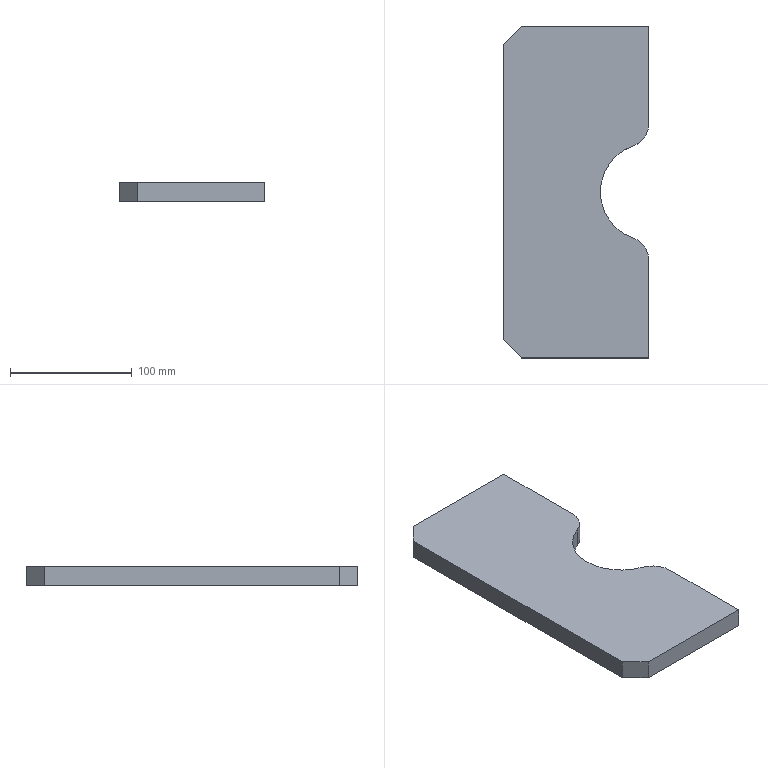Part | SolidWorks | features Extrusion 1 | 1 solid | 13 faces | box 120 x 273 x 16 mm | volume 478824 mm3 | plane 9 | cylinder 4 | commonest cylinder face diameters 40 x2 80 x2
STEP:
#1=CARTESIAN_POINT('',(80.,136.5,16.));
#2=VERTEX_POINT('',#1);
#3=CARTESIAN_POINT('',(106.667,174.212,16.));
#4=VERTEX_POINT('',#3);
#5=CARTESIAN_POINT('',(120.,136.5,16.));
#6=DIRECTION('',(0.,0.,-1.));
#7=DIRECTION('',(1.,0.,0.));
#8=AXIS2_PLACEMENT_3D('',#5,#6,#7);
#9=CIRCLE('',#8,40.);
#10=EDGE_CURVE('',#2,#4,#9,.T.);
#11=ORIENTED_EDGE('',*,*,#10,.F.);
#12=CARTESIAN_POINT('',(80.,136.5,0.));
#13=VERTEX_POINT('',#12);
#14=CARTESIAN_POINT('',(80.,136.5,16.));
#15=DIRECTION('',(0.,0.,-1.));
#16=VECTOR('',#15,1000.);
#17=LINE('',#14,#16);
#18=EDGE_CURVE('',#2,#13,#17,.T.);
#19=ORIENTED_EDGE('',*,*,#18,.T.);
#20=CARTESIAN_POINT('',(106.667,174.212,0.));
#21=VERTEX_POINT('',#20);
#22=CARTESIAN_POINT('',(120.,136.5,0.));
#23=DIRECTION('',(0.,0.,-1.));
#24=DIRECTION('',(1.,0.,0.));
#25=AXIS2_PLACEMENT_3D('',#22,#23,#24);
#26=CIRCLE('',#25,40.);
#27=EDGE_CURVE('',#13,#21,#26,.T.);
#28=ORIENTED_EDGE('',*,*,#27,.T.);
#29=CARTESIAN_POINT('',(106.667,174.212,16.));
#30=DIRECTION('',(0.,0.,-1.));
#31=VECTOR('',#30,1000.);
#32=LINE('',#29,#31);
#33=EDGE_CURVE('',#4,#21,#32,.T.);
#34=ORIENTED_EDGE('',*,*,#33,.F.);
#35=EDGE_LOOP('',(#11,#19,#28,#34));
#36=FACE_OUTER_BOUND('',#35,.T.);
#37=CARTESIAN_POINT('',(120.,136.5,16.));
#38=DIRECTION('',(0.,0.,-1.));
#39=DIRECTION('',(-1.,0.,0.));
#40=AXIS2_PLACEMENT_3D('',#37,#38,#39);
#41=CYLINDRICAL_SURFACE('',#40,40.);
#42=ADVANCED_FACE('',(#36),#41,.F.);
#43=CARTESIAN_POINT('',(120.,193.069,0.));
#44=VERTEX_POINT('',#43);
#45=CARTESIAN_POINT('',(120.,273.,0.));
#46=VERTEX_POINT('',#45);
#47=CARTESIAN_POINT('',(120.,193.069,0.));
#48=DIRECTION('',(0.,1.,0.));
#49=VECTOR('',#48,1000.);
#50=LINE('',#47,#49);
#51=EDGE_CURVE('',#44,#46,#50,.T.);
#52=ORIENTED_EDGE('',*,*,#51,.T.);
#53=CARTESIAN_POINT('',(120.,273.,16.));
#54=VERTEX_POINT('',#53);
#55=CARTESIAN_POINT('',(120.,273.,16.));
#56=DIRECTION('',(0.,0.,-1.));
#57=VECTOR('',#56,1000.);
#58=LINE('',#55,#57);
#59=EDGE_CURVE('',#54,#46,#58,.T.);
#60=ORIENTED_EDGE('',*,*,#59,.F.);
#61=CARTESIAN_POINT('',(120.,193.069,16.));
#62=VERTEX_POINT('',#61);
#63=CARTESIAN_POINT('',(120.,193.069,16.));
#64=DIRECTION('',(0.,1.,0.));
#65=VECTOR('',#64,1000.);
#66=LINE('',#63,#65);
#67=EDGE_CURVE('',#62,#54,#66,.T.);
#68=ORIENTED_EDGE('',*,*,#67,.F.);
#69=CARTESIAN_POINT('',(120.,193.069,16.));
#70=DIRECTION('',(0.,0.,-1.));
#71=VECTOR('',#70,1000.);
#72=LINE('',#69,#71);
#73=EDGE_CURVE('',#62,#44,#72,.T.);
#74=ORIENTED_EDGE('',*,*,#73,.T.);
#75=EDGE_LOOP('',(#52,#60,#68,#74));
#76=FACE_OUTER_BOUND('',#75,.T.);
#77=CARTESIAN_POINT('',(120.,193.069,16.));
#78=DIRECTION('',(-1.,0.,0.));
#79=DIRECTION('',(0.,0.,1.));
#80=AXIS2_PLACEMENT_3D('',#77,#78,#79);
#81=PLANE('',#80);
#82=ADVANCED_FACE('',(#76),#81,.F.);
#83=CARTESIAN_POINT('',(15.,273.,0.));
#84=VERTEX_POINT('',#83);
#85=CARTESIAN_POINT('',(15.,273.,0.));
#86=DIRECTION('',(-1.,0.,0.));
#87=VECTOR('',#86,1000.);
#88=LINE('',#85,#87);
#89=EDGE_CURVE('',#46,#84,#88,.T.);
#90=ORIENTED_EDGE('',*,*,#89,.T.);
#91=CARTESIAN_POINT('',(15.,273.,16.));
#92=VERTEX_POINT('',#91);
#93=CARTESIAN_POINT('',(15.,273.,16.));
#94=DIRECTION('',(0.,0.,-1.));
#95=VECTOR('',#94,1000.);
#96=LINE('',#93,#95);
#97=EDGE_CURVE('',#92,#84,#96,.T.);
#98=ORIENTED_EDGE('',*,*,#97,.F.);
#99=CARTESIAN_POINT('',(15.,273.,16.));
#100=DIRECTION('',(-1.,0.,0.));
#101=VECTOR('',#100,1000.);
#102=LINE('',#99,#101);
#103=EDGE_CURVE('',#54,#92,#102,.T.);
#104=ORIENTED_EDGE('',*,*,#103,.F.);
#105=ORIENTED_EDGE('',*,*,#59,.T.);
#106=EDGE_LOOP('',(#90,#98,#104,#105));
#107=FACE_OUTER_BOUND('',#106,.T.);
#108=CARTESIAN_POINT('',(15.,273.,16.));
#109=DIRECTION('',(0.,-1.,0.));
#110=DIRECTION('',(0.,0.,-1.));
#111=AXIS2_PLACEMENT_3D('',#108,#109,#110);
#112=PLANE('',#111);
#113=ADVANCED_FACE('',(#107),#112,.F.);
#114=CARTESIAN_POINT('',(0.,258.,0.));
#115=VERTEX_POINT('',#114);
#116=CARTESIAN_POINT('',(0.,258.,0.));
#117=DIRECTION('',(-0.7071,-0.7071,0.));
#118=VECTOR('',#117,1000.);
#119=LINE('',#116,#118);
#120=EDGE_CURVE('',#84,#115,#119,.T.);
#121=ORIENTED_EDGE('',*,*,#120,.T.);
#122=CARTESIAN_POINT('',(0.,258.,16.));
#123=VERTEX_POINT('',#122);
#124=CARTESIAN_POINT('',(0.,258.,16.));
#125=DIRECTION('',(0.,0.,-1.));
#126=VECTOR('',#125,1000.);
#127=LINE('',#124,#126);
#128=EDGE_CURVE('',#123,#115,#127,.T.);
#129=ORIENTED_EDGE('',*,*,#128,.F.);
#130=CARTESIAN_POINT('',(0.,258.,16.));
#131=DIRECTION('',(-0.7071,-0.7071,0.));
#132=VECTOR('',#131,1000.);
#133=LINE('',#130,#132);
#134=EDGE_CURVE('',#92,#123,#133,.T.);
#135=ORIENTED_EDGE('',*,*,#134,.F.);
#136=ORIENTED_EDGE('',*,*,#97,.T.);
#137=EDGE_LOOP('',(#121,#129,#135,#136));
#138=FACE_OUTER_BOUND('',#137,.T.);
#139=CARTESIAN_POINT('',(0.,258.,16.));
#140=DIRECTION('',(0.7071,-0.7071,0.));
#141=DIRECTION('',(0.7071,0.7071,0.));
#142=AXIS2_PLACEMENT_3D('',#139,#140,#141);
#143=PLANE('',#142);
#144=ADVANCED_FACE('',(#138),#143,.F.);
#145=CARTESIAN_POINT('',(0.,15.,0.));
#146=VERTEX_POINT('',#145);
#147=CARTESIAN_POINT('',(0.,15.,0.));
#148=DIRECTION('',(0.,-1.,0.));
#149=VECTOR('',#148,1000.);
#150=LINE('',#147,#149);
#151=EDGE_CURVE('',#115,#146,#150,.T.);
#152=ORIENTED_EDGE('',*,*,#151,.T.);
#153=CARTESIAN_POINT('',(0.,15.,16.));
#154=VERTEX_POINT('',#153);
#155=CARTESIAN_POINT('',(0.,15.,16.));
#156=DIRECTION('',(0.,0.,-1.));
#157=VECTOR('',#156,1000.);
#158=LINE('',#155,#157);
#159=EDGE_CURVE('',#154,#146,#158,.T.);
#160=ORIENTED_EDGE('',*,*,#159,.F.);
#161=CARTESIAN_POINT('',(0.,15.,16.));
#162=DIRECTION('',(0.,-1.,0.));
#163=VECTOR('',#162,1000.);
#164=LINE('',#161,#163);
#165=EDGE_CURVE('',#123,#154,#164,.T.);
#166=ORIENTED_EDGE('',*,*,#165,.F.);
#167=ORIENTED_EDGE('',*,*,#128,.T.);
#168=EDGE_LOOP('',(#152,#160,#166,#167));
#169=FACE_OUTER_BOUND('',#168,.T.);
#170=CARTESIAN_POINT('',(0.,15.,16.));
#171=DIRECTION('',(1.,0.,0.));
#172=DIRECTION('',(0.,0.,-1.));
#173=AXIS2_PLACEMENT_3D('',#170,#171,#172);
#174=PLANE('',#173);
#175=ADVANCED_FACE('',(#169),#174,.F.);
#176=CARTESIAN_POINT('',(15.,0.,0.));
#177=VERTEX_POINT('',#176);
#178=CARTESIAN_POINT('',(15.,0.,0.));
#179=DIRECTION('',(0.7071,-0.7071,0.));
#180=VECTOR('',#179,1000.);
#181=LINE('',#178,#180);
#182=EDGE_CURVE('',#146,#177,#181,.T.);
#183=ORIENTED_EDGE('',*,*,#182,.T.);
#184=CARTESIAN_POINT('',(15.,0.,16.));
#185=VERTEX_POINT('',#184);
#186=CARTESIAN_POINT('',(15.,0.,16.));
#187=DIRECTION('',(0.,0.,-1.));
#188=VECTOR('',#187,1000.);
#189=LINE('',#186,#188);
#190=EDGE_CURVE('',#185,#177,#189,.T.);
#191=ORIENTED_EDGE('',*,*,#190,.F.);
#192=CARTESIAN_POINT('',(15.,0.,16.));
#193=DIRECTION('',(0.7071,-0.7071,0.));
#194=VECTOR('',#193,1000.);
#195=LINE('',#192,#194);
#196=EDGE_CURVE('',#154,#185,#195,.T.);
#197=ORIENTED_EDGE('',*,*,#196,.F.);
#198=ORIENTED_EDGE('',*,*,#159,.T.);
#199=EDGE_LOOP('',(#183,#191,#197,#198));
#200=FACE_OUTER_BOUND('',#199,.T.);
#201=CARTESIAN_POINT('',(15.,0.,16.));
#202=DIRECTION('',(0.7071,0.7071,0.));
#203=DIRECTION('',(-0.7071,0.7071,0.));
#204=AXIS2_PLACEMENT_3D('',#201,#202,#203);
#205=PLANE('',#204);
#206=ADVANCED_FACE('',(#200),#205,.F.);
#207=CARTESIAN_POINT('',(120.,0.,0.));
#208=VERTEX_POINT('',#207);
#209=CARTESIAN_POINT('',(15.,0.,0.));
#210=DIRECTION('',(1.,0.,0.));
#211=VECTOR('',#210,1000.);
#212=LINE('',#209,#211);
#213=EDGE_CURVE('',#177,#208,#212,.T.);
#214=ORIENTED_EDGE('',*,*,#213,.T.);
#215=CARTESIAN_POINT('',(120.,0.,16.));
#216=VERTEX_POINT('',#215);
#217=CARTESIAN_POINT('',(120.,0.,16.));
#218=DIRECTION('',(0.,0.,-1.));
#219=VECTOR('',#218,1000.);
#220=LINE('',#217,#219);
#221=EDGE_CURVE('',#216,#208,#220,.T.);
#222=ORIENTED_EDGE('',*,*,#221,.F.);
#223=CARTESIAN_POINT('',(15.,0.,16.));
#224=DIRECTION('',(1.,0.,0.));
#225=VECTOR('',#224,1000.);
#226=LINE('',#223,#225);
#227=EDGE_CURVE('',#185,#216,#226,.T.);
#228=ORIENTED_EDGE('',*,*,#227,.F.);
#229=ORIENTED_EDGE('',*,*,#190,.T.);
#230=EDGE_LOOP('',(#214,#222,#228,#229));
#231=FACE_OUTER_BOUND('',#230,.T.);
#232=CARTESIAN_POINT('',(15.,0.,16.));
#233=DIRECTION('',(0.,1.,0.));
#234=DIRECTION('',(0.,0.,1.));
#235=AXIS2_PLACEMENT_3D('',#232,#233,#234);
#236=PLANE('',#235);
#237=ADVANCED_FACE('',(#231),#236,.F.);
#238=CARTESIAN_POINT('',(120.,79.931,0.));
#239=VERTEX_POINT('',#238);
#240=CARTESIAN_POINT('',(120.,0.,0.));
#241=DIRECTION('',(0.,1.,0.));
#242=VECTOR('',#241,1000.);
#243=LINE('',#240,#242);
#244=EDGE_CURVE('',#208,#239,#243,.T.);
#245=ORIENTED_EDGE('',*,*,#244,.T.);
#246=CARTESIAN_POINT('',(120.,79.931,16.));
#247=VERTEX_POINT('',#246);
#248=CARTESIAN_POINT('',(120.,79.931,16.));
#249=DIRECTION('',(0.,0.,-1.));
#250=VECTOR('',#249,1000.);
#251=LINE('',#248,#250);
#252=EDGE_CURVE('',#247,#239,#251,.T.);
#253=ORIENTED_EDGE('',*,*,#252,.F.);
#254=CARTESIAN_POINT('',(120.,0.,16.));
#255=DIRECTION('',(0.,1.,0.));
#256=VECTOR('',#255,1000.);
#257=LINE('',#254,#256);
#258=EDGE_CURVE('',#216,#247,#257,.T.);
#259=ORIENTED_EDGE('',*,*,#258,.F.);
#260=ORIENTED_EDGE('',*,*,#221,.T.);
#261=EDGE_LOOP('',(#245,#253,#259,#260));
#262=FACE_OUTER_BOUND('',#261,.T.);
#263=CARTESIAN_POINT('',(120.,0.,16.));
#264=DIRECTION('',(-1.,0.,0.));
#265=DIRECTION('',(0.,0.,1.));
#266=AXIS2_PLACEMENT_3D('',#263,#264,#265);
#267=PLANE('',#266);
#268=ADVANCED_FACE('',(#262),#267,.F.);
#269=CARTESIAN_POINT('',(106.667,98.788,0.));
#270=VERTEX_POINT('',#269);
#271=CARTESIAN_POINT('',(100.,79.931,0.));
#272=DIRECTION('',(0.,0.,1.));
#273=DIRECTION('',(1.,0.,0.));
#274=AXIS2_PLACEMENT_3D('',#271,#272,#273);
#275=CIRCLE('',#274,20.);
#276=EDGE_CURVE('',#239,#270,#275,.T.);
#277=ORIENTED_EDGE('',*,*,#276,.T.);
#278=CARTESIAN_POINT('',(106.667,98.788,16.));
#279=VERTEX_POINT('',#278);
#280=CARTESIAN_POINT('',(106.667,98.788,16.));
#281=DIRECTION('',(0.,0.,-1.));
#282=VECTOR('',#281,1000.);
#283=LINE('',#280,#282);
#284=EDGE_CURVE('',#279,#270,#283,.T.);
#285=ORIENTED_EDGE('',*,*,#284,.F.);
#286=CARTESIAN_POINT('',(100.,79.931,16.));
#287=DIRECTION('',(0.,0.,1.));
#288=DIRECTION('',(1.,0.,0.));
#289=AXIS2_PLACEMENT_3D('',#286,#287,#288);
#290=CIRCLE('',#289,20.);
#291=EDGE_CURVE('',#247,#279,#290,.T.);
#292=ORIENTED_EDGE('',*,*,#291,.F.);
#293=ORIENTED_EDGE('',*,*,#252,.T.);
#294=EDGE_LOOP('',(#277,#285,#292,#293));
#295=FACE_OUTER_BOUND('',#294,.T.);
#296=CARTESIAN_POINT('',(100.,79.931,16.));
#297=DIRECTION('',(0.,0.,-1.));
#298=DIRECTION('',(-1.,0.,0.));
#299=AXIS2_PLACEMENT_3D('',#296,#297,#298);
#300=CYLINDRICAL_SURFACE('',#299,20.);
#301=ADVANCED_FACE('',(#295),#300,.T.);
#302=ORIENTED_EDGE('',*,*,#18,.F.);
#303=CARTESIAN_POINT('',(120.,136.5,16.));
#304=DIRECTION('',(0.,0.,-1.));
#305=DIRECTION('',(1.,0.,0.));
#306=AXIS2_PLACEMENT_3D('',#303,#304,#305);
#307=CIRCLE('',#306,40.);
#308=EDGE_CURVE('',#279,#2,#307,.T.);
#309=ORIENTED_EDGE('',*,*,#308,.F.);
#310=ORIENTED_EDGE('',*,*,#284,.T.);
#311=CARTESIAN_POINT('',(120.,136.5,0.));
#312=DIRECTION('',(0.,0.,-1.));
#313=DIRECTION('',(1.,0.,0.));
#314=AXIS2_PLACEMENT_3D('',#311,#312,#313);
#315=CIRCLE('',#314,40.);
#316=EDGE_CURVE('',#270,#13,#315,.T.);
#317=ORIENTED_EDGE('',*,*,#316,.T.);
#318=EDGE_LOOP('',(#302,#309,#310,#317));
#319=FACE_OUTER_BOUND('',#318,.T.);
#320=CARTESIAN_POINT('',(120.,136.5,16.));
#321=DIRECTION('',(0.,0.,-1.));
#322=DIRECTION('',(-1.,0.,0.));
#323=AXIS2_PLACEMENT_3D('',#320,#321,#322);
#324=CYLINDRICAL_SURFACE('',#323,40.);
#325=ADVANCED_FACE('',(#319),#324,.F.);
#326=CARTESIAN_POINT('',(100.,193.069,0.));
#327=DIRECTION('',(0.,0.,1.));
#328=DIRECTION('',(-1.,0.,0.));
#329=AXIS2_PLACEMENT_3D('',#326,#327,#328);
#330=CIRCLE('',#329,20.);
#331=EDGE_CURVE('',#21,#44,#330,.T.);
#332=ORIENTED_EDGE('',*,*,#331,.T.);
#333=ORIENTED_EDGE('',*,*,#73,.F.);
#334=CARTESIAN_POINT('',(100.,193.069,16.));
#335=DIRECTION('',(0.,0.,1.));
#336=DIRECTION('',(-1.,0.,0.));
#337=AXIS2_PLACEMENT_3D('',#334,#335,#336);
#338=CIRCLE('',#337,20.);
#339=EDGE_CURVE('',#4,#62,#338,.T.);
#340=ORIENTED_EDGE('',*,*,#339,.F.);
#341=ORIENTED_EDGE('',*,*,#33,.T.);
#342=EDGE_LOOP('',(#332,#333,#340,#341));
#343=FACE_OUTER_BOUND('',#342,.T.);
#344=CARTESIAN_POINT('',(100.,193.069,16.));
#345=DIRECTION('',(0.,0.,-1.));
#346=DIRECTION('',(-1.,0.,0.));
#347=AXIS2_PLACEMENT_3D('',#344,#345,#346);
#348=CYLINDRICAL_SURFACE('',#347,20.);
#349=ADVANCED_FACE('',(#343),#348,.T.);
#350=ORIENTED_EDGE('',*,*,#67,.T.);
#351=ORIENTED_EDGE('',*,*,#103,.T.);
#352=ORIENTED_EDGE('',*,*,#134,.T.);
#353=ORIENTED_EDGE('',*,*,#165,.T.);
#354=ORIENTED_EDGE('',*,*,#196,.T.);
#355=ORIENTED_EDGE('',*,*,#227,.T.);
#356=ORIENTED_EDGE('',*,*,#258,.T.);
#357=ORIENTED_EDGE('',*,*,#291,.T.);
#358=ORIENTED_EDGE('',*,*,#308,.T.);
#359=ORIENTED_EDGE('',*,*,#10,.T.);
#360=ORIENTED_EDGE('',*,*,#339,.T.);
#361=EDGE_LOOP('',(#350,#351,#352,#353,#354,#355,#356,#357,#358,#359,#360));
#362=FACE_OUTER_BOUND('',#361,.T.);
#363=CARTESIAN_POINT('',(100.,79.931,16.));
#364=DIRECTION('',(0.,0.,1.));
#365=DIRECTION('',(1.,0.,0.));
#366=AXIS2_PLACEMENT_3D('',#363,#364,#365);
#367=PLANE('',#366);
#368=ADVANCED_FACE('',(#362),#367,.T.);
#369=ORIENTED_EDGE('',*,*,#51,.F.);
#370=ORIENTED_EDGE('',*,*,#331,.F.);
#371=ORIENTED_EDGE('',*,*,#27,.F.);
#372=ORIENTED_EDGE('',*,*,#316,.F.);
#373=ORIENTED_EDGE('',*,*,#276,.F.);
#374=ORIENTED_EDGE('',*,*,#244,.F.);
#375=ORIENTED_EDGE('',*,*,#213,.F.);
#376=ORIENTED_EDGE('',*,*,#182,.F.);
#377=ORIENTED_EDGE('',*,*,#151,.F.);
#378=ORIENTED_EDGE('',*,*,#120,.F.);
#379=ORIENTED_EDGE('',*,*,#89,.F.);
#380=EDGE_LOOP('',(#369,#370,#371,#372,#373,#374,#375,#376,#377,#378,#379));
#381=FACE_OUTER_BOUND('',#380,.T.);
#382=CARTESIAN_POINT('',(100.,79.931,0.));
#383=DIRECTION('',(0.,0.,1.));
#384=DIRECTION('',(1.,0.,0.));
#385=AXIS2_PLACEMENT_3D('',#382,#383,#384);
#386=PLANE('',#385);
#387=ADVANCED_FACE('',(#381),#386,.F.);
#388=CLOSED_SHELL('',(#42,#82,#113,#144,#175,#206,#237,#268,#301,#325,#349,#368,#387));
#389=MANIFOLD_SOLID_BREP('',#388);
#390=CARTESIAN_POINT('',(0.,0.,0.));
#391=DIRECTION('',(0.,0.,1.));
#392=DIRECTION('',(1.,0.,0.));
#393=AXIS2_PLACEMENT_3D('',#390,#391,#392);
#394=(LENGTH_UNIT()NAMED_UNIT(*)SI_UNIT(.MILLI.,.METRE.));
#395=UNCERTAINTY_MEASURE_WITH_UNIT(LENGTH_MEASURE(0.00001),#394,'','');
#396=(NAMED_UNIT(*)PLANE_ANGLE_UNIT()SI_UNIT($,.RADIAN.));
#397=(NAMED_UNIT(*)SI_UNIT($,.STERADIAN.)SOLID_ANGLE_UNIT());
#398=(GEOMETRIC_REPRESENTATION_CONTEXT(3)GLOBAL_UNCERTAINTY_ASSIGNED_CONTEXT((#395))GLOBAL_UNIT_ASSIGNED_CONTEXT((#394,#396,#397))REPRESENTATION_CONTEXT('',''));
#399=ADVANCED_BREP_SHAPE_REPRESENTATION('',(#389,#393),#398);